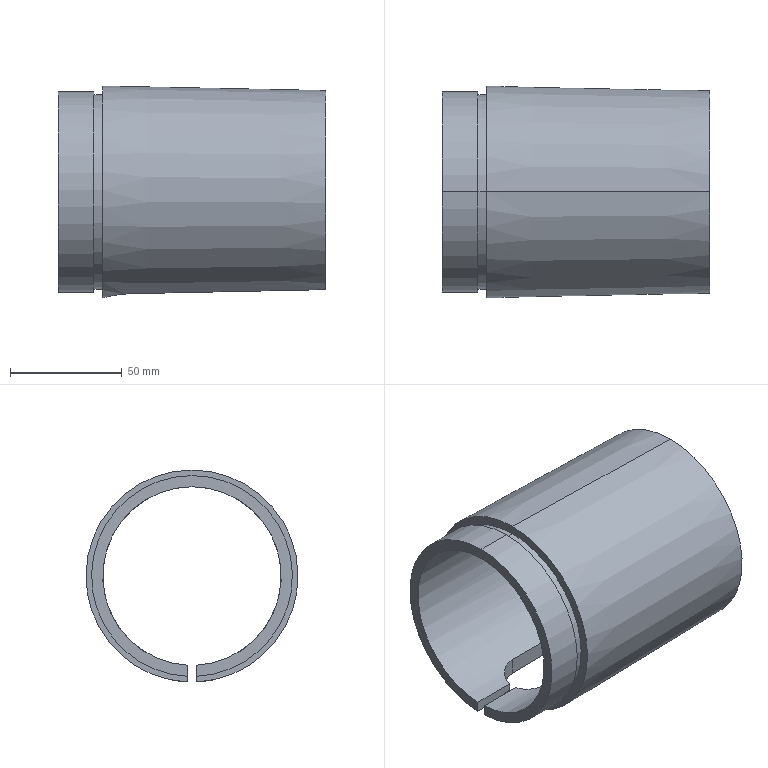Part | STEP file | Taper sleeve | 1 solid | 18 faces | box 120 x 95 x 94.958 mm | volume 185425 mm3 | cylinder 8 | plane 8 | cone 2 | commonest cylinder face diameters 25 x2 80 x2 87 x2 90 x2